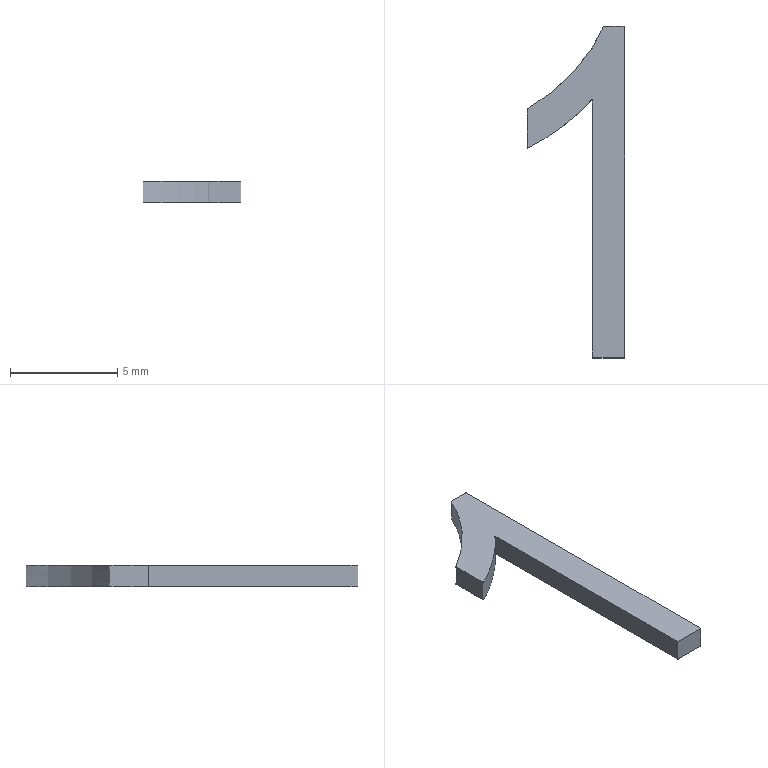Part | STEP file | lll_id974_x_t | 1 solid | 3 faces | box 4.557 x 15.502 x 1 mm | volume 21.922 mm3 | plane 2 | other 1